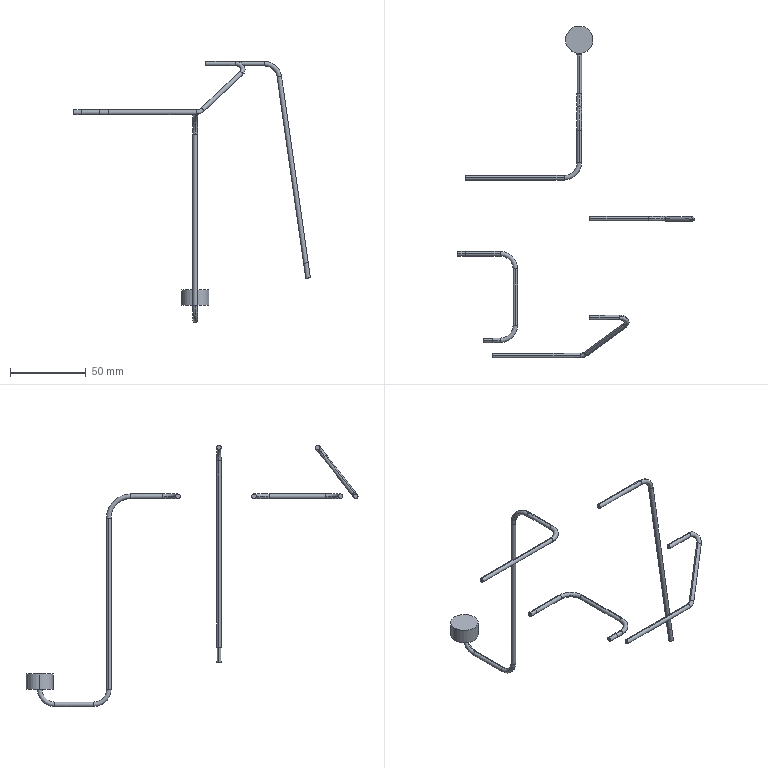Part | SolidWorks | features 3DProfileFeature 5, Sweep 4, ICE 1 | 4 solids | 59 faces | box 155.715 x 218.5 x 171.95 mm | volume 7637 mm3 | cylinder 32 | torus 18 | plane 9 | commonest cylinder face diameters 3 x30 18 x2